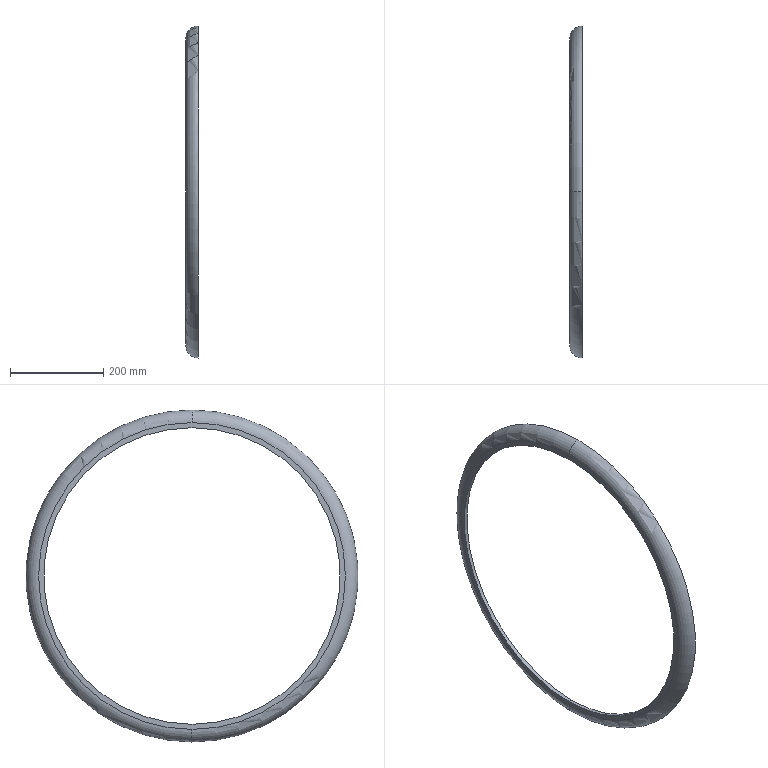Part | SolidWorks | features Revolution 1 | 1 solid | 9 faces | box 27 x 711 x 711 mm | volume 802010 mm3 | torus 4 | plane 3 | cylinder 2 | commonest cylinder face diameters 635 x2
STEP:
#1=CARTESIAN_POINT('',(0.,0.,-347.5));
#2=VERTEX_POINT('',#1);
#3=CARTESIAN_POINT('',(0.,0.,347.5));
#4=VERTEX_POINT('',#3);
#5=CARTESIAN_POINT('',(0.,0.,0.));
#6=DIRECTION('',(-1.,0.,0.));
#7=DIRECTION('',(0.,0.,1.));
#8=AXIS2_PLACEMENT_3D('',#5,#6,#7);
#9=CIRCLE('',#8,347.5);
#10=EDGE_CURVE('',#2,#4,#9,.T.);
#11=ORIENTED_EDGE('',*,*,#10,.F.);
#12=CARTESIAN_POINT('',(-19.,0.,-328.5));
#13=VERTEX_POINT('',#12);
#14=CARTESIAN_POINT('',(0.,0.,-328.5));
#15=DIRECTION('',(0.,1.,0.));
#16=DIRECTION('',(0.,0.,1.));
#17=AXIS2_PLACEMENT_3D('',#14,#15,#16);
#18=CIRCLE('',#17,19.);
#19=EDGE_CURVE('',#2,#13,#18,.T.);
#20=ORIENTED_EDGE('',*,*,#19,.T.);
#21=CARTESIAN_POINT('',(-19.,0.,328.5));
#22=VERTEX_POINT('',#21);
#23=CARTESIAN_POINT('',(-19.,0.,0.));
#24=DIRECTION('',(-1.,0.,0.));
#25=DIRECTION('',(0.,0.,1.));
#26=AXIS2_PLACEMENT_3D('',#23,#24,#25);
#27=CIRCLE('',#26,328.5);
#28=EDGE_CURVE('',#13,#22,#27,.T.);
#29=ORIENTED_EDGE('',*,*,#28,.T.);
#30=CARTESIAN_POINT('',(0.,0.,328.5));
#31=DIRECTION('',(0.,-1.,0.));
#32=DIRECTION('',(0.,0.,-1.));
#33=AXIS2_PLACEMENT_3D('',#30,#31,#32);
#34=CIRCLE('',#33,19.);
#35=EDGE_CURVE('',#4,#22,#34,.T.);
#36=ORIENTED_EDGE('',*,*,#35,.F.);
#37=EDGE_LOOP('',(#11,#20,#29,#36));
#38=FACE_OUTER_BOUND('',#37,.T.);
#39=CARTESIAN_POINT('',(0.,0.,0.));
#40=DIRECTION('',(-1.,0.,0.));
#41=DIRECTION('',(0.,0.,1.));
#42=AXIS2_PLACEMENT_3D('',#39,#40,#41);
#43=TOROIDAL_SURFACE('',#42,328.5,19.);
#44=ADVANCED_FACE('',(#38),#43,.F.);
#45=CARTESIAN_POINT('',(-19.,0.,-317.5));
#46=VERTEX_POINT('',#45);
#47=CARTESIAN_POINT('',(-19.,0.,317.5));
#48=VERTEX_POINT('',#47);
#49=CARTESIAN_POINT('',(-19.,0.,0.));
#50=DIRECTION('',(-1.,0.,0.));
#51=DIRECTION('',(0.,0.,1.));
#52=AXIS2_PLACEMENT_3D('',#49,#50,#51);
#53=CIRCLE('',#52,317.5);
#54=EDGE_CURVE('',#46,#48,#53,.T.);
#55=ORIENTED_EDGE('',*,*,#54,.F.);
#56=CARTESIAN_POINT('',(-27.,0.,-317.5));
#57=VERTEX_POINT('',#56);
#58=CARTESIAN_POINT('',(-257.767,0.,-317.5));
#59=DIRECTION('',(-1.,0.,0.));
#60=VECTOR('',#59,1000.);
#61=LINE('',#58,#60);
#62=EDGE_CURVE('',#46,#57,#61,.T.);
#63=ORIENTED_EDGE('',*,*,#62,.T.);
#64=CARTESIAN_POINT('',(-27.,0.,317.5));
#65=VERTEX_POINT('',#64);
#66=CARTESIAN_POINT('',(-27.,0.,0.));
#67=DIRECTION('',(-1.,0.,0.));
#68=DIRECTION('',(0.,0.,1.));
#69=AXIS2_PLACEMENT_3D('',#66,#67,#68);
#70=CIRCLE('',#69,317.5);
#71=EDGE_CURVE('',#57,#65,#70,.T.);
#72=ORIENTED_EDGE('',*,*,#71,.T.);
#73=CARTESIAN_POINT('',(-257.767,0.,317.5));
#74=DIRECTION('',(-1.,0.,0.));
#75=VECTOR('',#74,1000.);
#76=LINE('',#73,#75);
#77=EDGE_CURVE('',#48,#65,#76,.T.);
#78=ORIENTED_EDGE('',*,*,#77,.F.);
#79=EDGE_LOOP('',(#55,#63,#72,#78));
#80=FACE_OUTER_BOUND('',#79,.T.);
#81=CARTESIAN_POINT('',(-257.767,0.,0.));
#82=DIRECTION('',(-1.,0.,0.));
#83=DIRECTION('',(0.,0.,1.));
#84=AXIS2_PLACEMENT_3D('',#81,#82,#83);
#85=CYLINDRICAL_SURFACE('',#84,317.5);
#86=ADVANCED_FACE('',(#80),#85,.F.);
#87=CARTESIAN_POINT('',(0.,0.,355.5));
#88=VERTEX_POINT('',#87);
#89=CARTESIAN_POINT('',(0.,0.,-355.5));
#90=VERTEX_POINT('',#89);
#91=CARTESIAN_POINT('',(0.,0.,0.));
#92=DIRECTION('',(-1.,0.,0.));
#93=DIRECTION('',(0.,0.,1.));
#94=AXIS2_PLACEMENT_3D('',#91,#92,#93);
#95=CIRCLE('',#94,355.5);
#96=EDGE_CURVE('',#88,#90,#95,.T.);
#97=ORIENTED_EDGE('',*,*,#96,.T.);
#98=CARTESIAN_POINT('',(-27.,0.,-328.5));
#99=VERTEX_POINT('',#98);
#100=CARTESIAN_POINT('',(0.,0.,-328.5));
#101=DIRECTION('',(0.,1.,0.));
#102=DIRECTION('',(0.,0.,1.));
#103=AXIS2_PLACEMENT_3D('',#100,#101,#102);
#104=CIRCLE('',#103,27.);
#105=EDGE_CURVE('',#90,#99,#104,.T.);
#106=ORIENTED_EDGE('',*,*,#105,.T.);
#107=CARTESIAN_POINT('',(-27.,0.,328.5));
#108=VERTEX_POINT('',#107);
#109=CARTESIAN_POINT('',(-27.,0.,0.));
#110=DIRECTION('',(-1.,0.,0.));
#111=DIRECTION('',(0.,0.,1.));
#112=AXIS2_PLACEMENT_3D('',#109,#110,#111);
#113=CIRCLE('',#112,328.5);
#114=EDGE_CURVE('',#108,#99,#113,.T.);
#115=ORIENTED_EDGE('',*,*,#114,.F.);
#116=CARTESIAN_POINT('',(0.,0.,328.5));
#117=DIRECTION('',(0.,-1.,0.));
#118=DIRECTION('',(0.,0.,-1.));
#119=AXIS2_PLACEMENT_3D('',#116,#117,#118);
#120=CIRCLE('',#119,27.);
#121=EDGE_CURVE('',#88,#108,#120,.T.);
#122=ORIENTED_EDGE('',*,*,#121,.F.);
#123=EDGE_LOOP('',(#97,#106,#115,#122));
#124=FACE_OUTER_BOUND('',#123,.T.);
#125=CARTESIAN_POINT('',(0.,0.,0.));
#126=DIRECTION('',(-1.,0.,0.));
#127=DIRECTION('',(0.,0.,1.));
#128=AXIS2_PLACEMENT_3D('',#125,#126,#127);
#129=TOROIDAL_SURFACE('',#128,328.5,27.);
#130=ADVANCED_FACE('',(#124),#129,.T.);
#131=ORIENTED_EDGE('',*,*,#105,.F.);
#132=CARTESIAN_POINT('',(0.,0.,0.));
#133=DIRECTION('',(-1.,0.,0.));
#134=DIRECTION('',(0.,0.,1.));
#135=AXIS2_PLACEMENT_3D('',#132,#133,#134);
#136=CIRCLE('',#135,355.5);
#137=EDGE_CURVE('',#90,#88,#136,.T.);
#138=ORIENTED_EDGE('',*,*,#137,.T.);
#139=ORIENTED_EDGE('',*,*,#121,.T.);
#140=CARTESIAN_POINT('',(-27.,0.,0.));
#141=DIRECTION('',(-1.,0.,0.));
#142=DIRECTION('',(0.,0.,1.));
#143=AXIS2_PLACEMENT_3D('',#140,#141,#142);
#144=CIRCLE('',#143,328.5);
#145=EDGE_CURVE('',#99,#108,#144,.T.);
#146=ORIENTED_EDGE('',*,*,#145,.F.);
#147=EDGE_LOOP('',(#131,#138,#139,#146));
#148=FACE_OUTER_BOUND('',#147,.T.);
#149=CARTESIAN_POINT('',(0.,0.,0.));
#150=DIRECTION('',(-1.,0.,0.));
#151=DIRECTION('',(0.,0.,1.));
#152=AXIS2_PLACEMENT_3D('',#149,#150,#151);
#153=TOROIDAL_SURFACE('',#152,328.5,27.);
#154=ADVANCED_FACE('',(#148),#153,.T.);
#155=CARTESIAN_POINT('',(-27.,0.,0.));
#156=DIRECTION('',(-1.,0.,0.));
#157=DIRECTION('',(0.,0.,1.));
#158=AXIS2_PLACEMENT_3D('',#155,#156,#157);
#159=CIRCLE('',#158,317.5);
#160=EDGE_CURVE('',#65,#57,#159,.T.);
#161=ORIENTED_EDGE('',*,*,#160,.F.);
#162=ORIENTED_EDGE('',*,*,#71,.F.);
#163=EDGE_LOOP('',(#161,#162));
#164=FACE_BOUND('',#163,.T.);
#165=ORIENTED_EDGE('',*,*,#114,.T.);
#166=ORIENTED_EDGE('',*,*,#145,.T.);
#167=EDGE_LOOP('',(#165,#166));
#168=FACE_OUTER_BOUND('',#167,.T.);
#169=CARTESIAN_POINT('',(-27.,328.5,0.));
#170=DIRECTION('',(1.,0.,0.));
#171=DIRECTION('',(0.,0.,-1.));
#172=AXIS2_PLACEMENT_3D('',#169,#170,#171);
#173=PLANE('',#172);
#174=ADVANCED_FACE('',(#164,#168),#173,.F.);
#175=ORIENTED_EDGE('',*,*,#62,.F.);
#176=CARTESIAN_POINT('',(-19.,0.,0.));
#177=DIRECTION('',(-1.,0.,0.));
#178=DIRECTION('',(0.,0.,1.));
#179=AXIS2_PLACEMENT_3D('',#176,#177,#178);
#180=CIRCLE('',#179,317.5);
#181=EDGE_CURVE('',#48,#46,#180,.T.);
#182=ORIENTED_EDGE('',*,*,#181,.F.);
#183=ORIENTED_EDGE('',*,*,#77,.T.);
#184=ORIENTED_EDGE('',*,*,#160,.T.);
#185=EDGE_LOOP('',(#175,#182,#183,#184));
#186=FACE_OUTER_BOUND('',#185,.T.);
#187=CARTESIAN_POINT('',(-257.767,0.,0.));
#188=DIRECTION('',(-1.,0.,0.));
#189=DIRECTION('',(0.,0.,1.));
#190=AXIS2_PLACEMENT_3D('',#187,#188,#189);
#191=CYLINDRICAL_SURFACE('',#190,317.5);
#192=ADVANCED_FACE('',(#186),#191,.F.);
#193=CARTESIAN_POINT('',(-19.,0.,0.));
#194=DIRECTION('',(-1.,0.,0.));
#195=DIRECTION('',(0.,0.,1.));
#196=AXIS2_PLACEMENT_3D('',#193,#194,#195);
#197=CIRCLE('',#196,328.5);
#198=EDGE_CURVE('',#22,#13,#197,.T.);
#199=ORIENTED_EDGE('',*,*,#198,.F.);
#200=ORIENTED_EDGE('',*,*,#28,.F.);
#201=EDGE_LOOP('',(#199,#200));
#202=FACE_OUTER_BOUND('',#201,.T.);
#203=ORIENTED_EDGE('',*,*,#181,.T.);
#204=ORIENTED_EDGE('',*,*,#54,.T.);
#205=EDGE_LOOP('',(#203,#204));
#206=FACE_BOUND('',#205,.T.);
#207=CARTESIAN_POINT('',(-19.,328.5,0.));
#208=DIRECTION('',(-1.,0.,0.));
#209=DIRECTION('',(0.,0.,1.));
#210=AXIS2_PLACEMENT_3D('',#207,#208,#209);
#211=PLANE('',#210);
#212=ADVANCED_FACE('',(#202,#206),#211,.F.);
#213=ORIENTED_EDGE('',*,*,#19,.F.);
#214=CARTESIAN_POINT('',(0.,0.,0.));
#215=DIRECTION('',(-1.,0.,0.));
#216=DIRECTION('',(0.,0.,1.));
#217=AXIS2_PLACEMENT_3D('',#214,#215,#216);
#218=CIRCLE('',#217,347.5);
#219=EDGE_CURVE('',#4,#2,#218,.T.);
#220=ORIENTED_EDGE('',*,*,#219,.F.);
#221=ORIENTED_EDGE('',*,*,#35,.T.);
#222=ORIENTED_EDGE('',*,*,#198,.T.);
#223=EDGE_LOOP('',(#213,#220,#221,#222));
#224=FACE_OUTER_BOUND('',#223,.T.);
#225=CARTESIAN_POINT('',(0.,0.,0.));
#226=DIRECTION('',(-1.,0.,0.));
#227=DIRECTION('',(0.,0.,1.));
#228=AXIS2_PLACEMENT_3D('',#225,#226,#227);
#229=TOROIDAL_SURFACE('',#228,328.5,19.);
#230=ADVANCED_FACE('',(#224),#229,.F.);
#231=ORIENTED_EDGE('',*,*,#96,.F.);
#232=ORIENTED_EDGE('',*,*,#137,.F.);
#233=EDGE_LOOP('',(#231,#232));
#234=FACE_OUTER_BOUND('',#233,.T.);
#235=ORIENTED_EDGE('',*,*,#219,.T.);
#236=ORIENTED_EDGE('',*,*,#10,.T.);
#237=EDGE_LOOP('',(#235,#236));
#238=FACE_BOUND('',#237,.T.);
#239=CARTESIAN_POINT('',(0.,355.5,0.));
#240=DIRECTION('',(-1.,0.,0.));
#241=DIRECTION('',(0.,0.,1.));
#242=AXIS2_PLACEMENT_3D('',#239,#240,#241);
#243=PLANE('',#242);
#244=ADVANCED_FACE('',(#234,#238),#243,.F.);
#245=CLOSED_SHELL('',(#44,#86,#130,#154,#174,#192,#212,#230,#244));
#246=MANIFOLD_SOLID_BREP('',#245);
#247=CARTESIAN_POINT('',(0.,0.,0.));
#248=DIRECTION('',(0.,0.,1.));
#249=DIRECTION('',(1.,0.,0.));
#250=AXIS2_PLACEMENT_3D('',#247,#248,#249);
#251=(LENGTH_UNIT()NAMED_UNIT(*)SI_UNIT(.MILLI.,.METRE.));
#252=UNCERTAINTY_MEASURE_WITH_UNIT(LENGTH_MEASURE(0.00001),#251,'','');
#253=(NAMED_UNIT(*)PLANE_ANGLE_UNIT()SI_UNIT($,.RADIAN.));
#254=(NAMED_UNIT(*)SI_UNIT($,.STERADIAN.)SOLID_ANGLE_UNIT());
#255=(GEOMETRIC_REPRESENTATION_CONTEXT(3)GLOBAL_UNCERTAINTY_ASSIGNED_CONTEXT((#252))GLOBAL_UNIT_ASSIGNED_CONTEXT((#251,#253,#254))REPRESENTATION_CONTEXT('',''));
#256=ADVANCED_BREP_SHAPE_REPRESENTATION('',(#246,#250),#255);